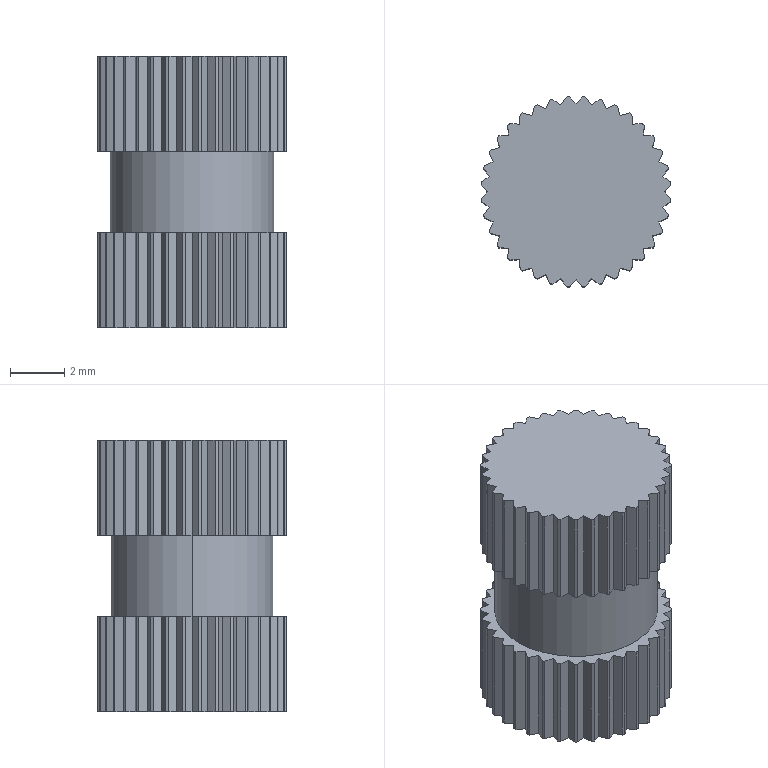Part | NX | features solid 2 | 1 solid | 226 faces | box 6.982 x 6.982 x 10 mm | volume 216.895 mm3 | plane 148 | cylinder 76 | cone 2 | commonest cylinder face diameters 7 x72 4.2 x2 6 x2